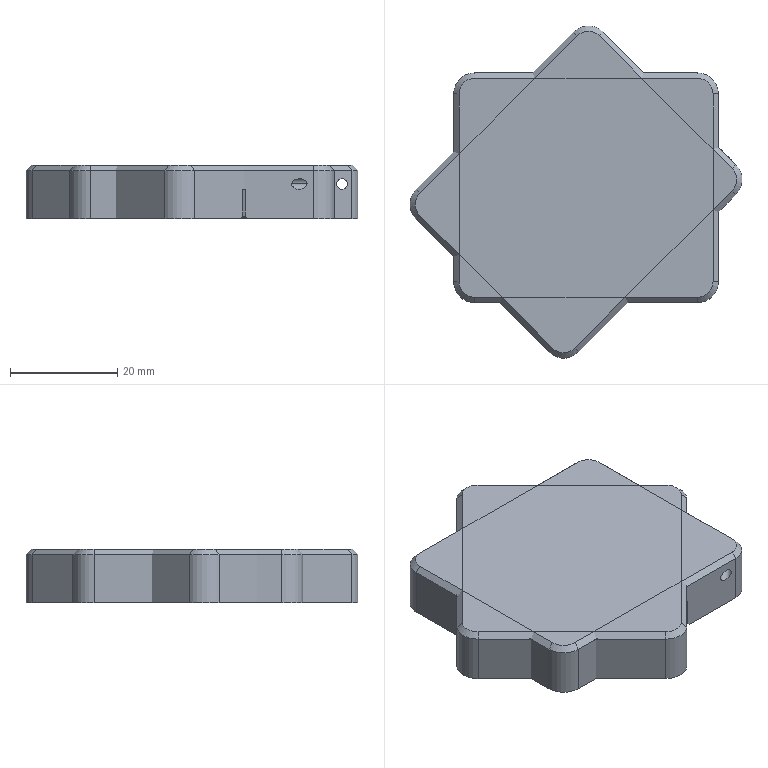NC program | NX | posted with a generic post | part box 61.954 x 61.954 x 10 mm
Lines 2952 to 3041 of 3041:
(PLANAR_MILL_3 , TOOL : D8倒角刀)
N5860 T05 M6
N5862 G54
N5864 G17 G0 G90 X14.798 Y22.189 B0. C0. S3500 M3
N5866 G43 Z30. H5
N5868 Z1.5
N5870 G94 G1 Z-1.5 F800.
N5872 X10.909 Y18.3
N5874 X7.472 Y14.863
N5876 G2 X5.351 Y14.863 R1.5
N5878 G1 X2.23 Y17.984
N5880 G3 X-1.436 Y19.067 R4.
N5882 X21.717 Y-4.086 R-19.5
N5884 X20.634 Y-0.42 R4.
N5886 G1 X17.513 Y2.701
N5888 G2 X17.513 Y4.822 R1.5
N5890 G1 X20.95 Y8.259
N5892 X24.839 Y12.148
N5894 Z1.5
N5896 G0 Z30.
(PLANAR_MILL_3_COPY , TOOL : D8倒角刀)
N5898 X19.111 Y12.219
N5900 Z1.5
N5902 G1 Z-1.5
N5904 X23.001 Y8.33
N5906 X31.663 Y-0.332
N5908 G2 X31.663 Y-8.012 R5.43
N5910 G1 X6.914 Y-32.76
N5912 G2 X-0.765 Y-32.76 R5.43
N5914 G1 X-30.11 Y-3.415
N5916 G2 X-30.11 Y4.264 R5.43
N5918 G1 X-5.362 Y29.013
N5920 G2 X2.318 Y29.013 R5.43
N5922 G1 X10.98 Y20.351
N5924 X14.869 Y16.461
N5926 Z1.5
N5928 G0 Z30.
(PLANAR_MILL_3_COPY_COPY , TOOL : D8倒角刀)
N5930 X27.469 Y-3.818
N5932 Z0.5
N5934 G1 Z-1.5
N5936 X27.116 Y-4.172
N5938 G3 X27.116 Y-4.879 R0.5
N5940 X28.53 Y-4.879 R1.
N5942 X27.116 Y-4.879 R-1.
N5944 X27.823 Y-4.879 R0.5
N5946 G1 X28.176 Y-4.526
N5948 Z0.5
N5950 G0 Z30.
N5952 X3.428 Y-29.274
N5954 Z0.5
N5956 G1 Z-1.5
N5958 X3.781 Y-28.921
N5960 G3 X3.781 Y-28.214 R0.5
N5962 X2.367 Y-28.214 R1.
N5964 X3.781 Y-28.214 R-1.
N5966 X3.074 Y-28.214 R0.5
N5968 G1 X2.721 Y-28.567
N5970 Z0.5
N5972 G0 Z30.
N5974 X-25.917 Y0.071
N5976 Z0.5
N5978 G1 Z-1.5
N5980 X-25.564 Y0.424
N5982 G3 X-25.564 Y1.131 R0.5
N5984 X-26.978 Y1.131 R1.
N5986 X-25.564 Y1.131 R-1.
N5988 X-26.271 Y1.131 R0.5
N5990 G1 X-26.624 Y0.778
N5992 Z0.5
N5994 G0 Z30.
N5996 X-1.876 Y25.526
N5998 Z0.5
N6000 G1 Z-1.5
N6002 X-2.229 Y25.173
N6004 G3 X-2.229 Y24.466 R0.5
N6006 X-0.815 Y24.466 R1.
N6008 X-2.229 Y24.466 R-1.
N6010 X-1.522 Y24.466 R0.5
N6012 G1 X-1.169 Y24.819
N6014 Z0.5
N6016 G0 Z30.
N6018 M5
N6020 M2